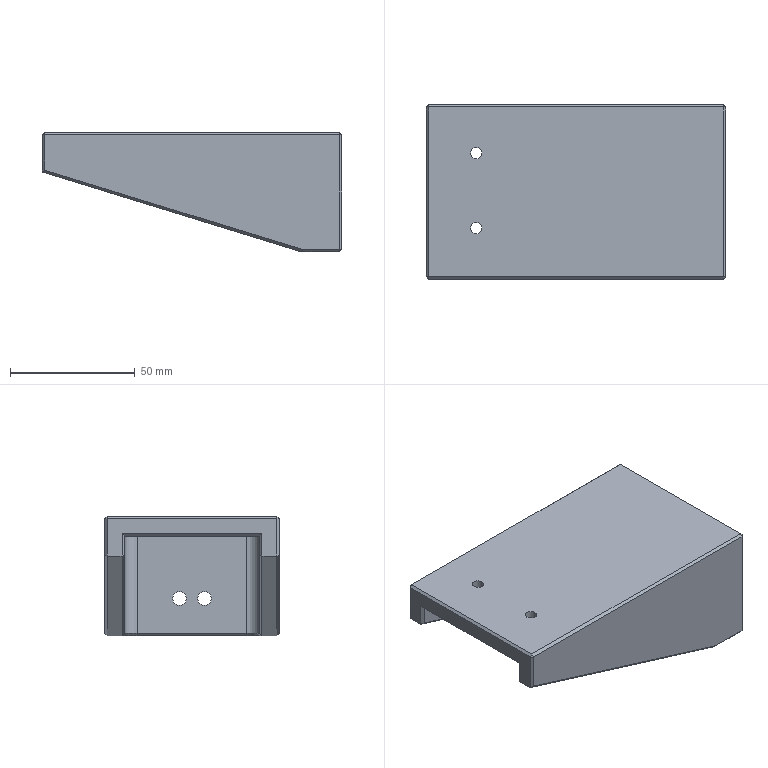Part | 1 solid | 47 faces | box 120 x 70 x 48 mm | volume 133864 mm3 | plane 39 | cylinder 6 | cone 2 | commonest cylinder face diameters 4.5 x2 5.5 x2 10 x2
STEP:
#1=CARTESIAN_POINT('',(44.15,35.,-47.));
#2=VERTEX_POINT('',#1);
#3=CARTESIAN_POINT('',(44.,34.,-48.));
#4=VERTEX_POINT('',#3);
#5=CARTESIAN_POINT('',(44.15,35.,-47.));
#6=CARTESIAN_POINT('',(44.,34.,-48.));
#7=B_SPLINE_CURVE_WITH_KNOTS('',1,(#5,#6),.UNSPECIFIED.,.F.,.F.,(2,2),(-0.7111,0.7111),.UNSPECIFIED.);
#8=EDGE_CURVE('',#2,#4,#7,.T.);
#9=ORIENTED_EDGE('',*,*,#8,.F.);
#10=CARTESIAN_POINT('',(59.,35.,-47.));
#11=VERTEX_POINT('',#10);
#12=CARTESIAN_POINT('',(51.575,35.,-47.));
#13=DIRECTION('',(-1.,0.,0.));
#14=VECTOR('',#13,1000.);
#15=LINE('',#12,#14);
#16=EDGE_CURVE('',#11,#2,#15,.T.);
#17=ORIENTED_EDGE('',*,*,#16,.F.);
#18=CARTESIAN_POINT('',(59.,34.,-48.));
#19=VERTEX_POINT('',#18);
#20=CARTESIAN_POINT('',(59.,34.5,-47.5));
#21=DIRECTION('',(0.,-0.7071,-0.7071));
#22=VECTOR('',#21,1000.);
#23=LINE('',#20,#22);
#24=EDGE_CURVE('',#11,#19,#23,.T.);
#25=ORIENTED_EDGE('',*,*,#24,.T.);
#26=CARTESIAN_POINT('',(51.5,34.,-48.));
#27=DIRECTION('',(-1.,0.,0.));
#28=VECTOR('',#27,1000.);
#29=LINE('',#26,#28);
#30=EDGE_CURVE('',#19,#4,#29,.T.);
#31=ORIENTED_EDGE('',*,*,#30,.T.);
#32=EDGE_LOOP('',(#9,#17,#25,#31));
#33=FACE_BOUND('',#32,.T.);
#34=CARTESIAN_POINT('',(-0.5,35.,-47.));
#35=DIRECTION('',(0.,-0.7071,0.7071));
#36=DIRECTION('',(-1.,0.,0.));
#37=AXIS2_PLACEMENT_3D('',#34,#35,#36);
#38=PLANE('',#37);
#39=ADVANCED_FACE('',(#33),#38,.F.);
#40=ORIENTED_EDGE('',*,*,#8,.T.);
#41=CARTESIAN_POINT('',(-60.,34.,-16.));
#42=VERTEX_POINT('',#41);
#43=CARTESIAN_POINT('',(-8.,34.,-32.));
#44=DIRECTION('',(-0.9558,0.,0.2941));
#45=VECTOR('',#44,1000.);
#46=LINE('',#43,#45);
#47=EDGE_CURVE('',#4,#42,#46,.T.);
#48=ORIENTED_EDGE('',*,*,#47,.T.);
#49=CARTESIAN_POINT('',(-59.,35.,-15.261));
#50=VERTEX_POINT('',#49);
#51=CARTESIAN_POINT('',(-59.,35.,-15.261));
#52=CARTESIAN_POINT('',(-60.,34.,-16.));
#53=B_SPLINE_CURVE_WITH_KNOTS('',1,(#51,#52),.UNSPECIFIED.,.F.,.F.,(2,2),(-0.7977,0.7977),.UNSPECIFIED.);
#54=EDGE_CURVE('',#50,#42,#53,.T.);
#55=ORIENTED_EDGE('',*,*,#54,.F.);
#56=CARTESIAN_POINT('',(-7.425,35.,-31.131));
#57=DIRECTION('',(-0.9558,0.,0.2941));
#58=VECTOR('',#57,1000.);
#59=LINE('',#56,#58);
#60=EDGE_CURVE('',#2,#50,#59,.T.);
#61=ORIENTED_EDGE('',*,*,#60,.F.);
#62=EDGE_LOOP('',(#40,#48,#55,#61));
#63=FACE_BOUND('',#62,.T.);
#64=CARTESIAN_POINT('',(-3.219,34.,-33.471));
#65=DIRECTION('',(-0.208,0.7071,-0.6758));
#66=DIRECTION('',(-0.9558,0.,0.2941));
#67=AXIS2_PLACEMENT_3D('',#64,#65,#66);
#68=PLANE('',#67);
#69=ADVANCED_FACE('',(#63),#68,.T.);
#70=CARTESIAN_POINT('',(-60.,34.,-1.));
#71=VERTEX_POINT('',#70);
#72=CARTESIAN_POINT('',(-60.,34.,-8.5));
#73=DIRECTION('',(0.,0.,-1.));
#74=VECTOR('',#73,1000.);
#75=LINE('',#72,#74);
#76=EDGE_CURVE('',#71,#42,#75,.T.);
#77=ORIENTED_EDGE('',*,*,#76,.F.);
#78=CARTESIAN_POINT('',(-59.,35.,-1.));
#79=VERTEX_POINT('',#78);
#80=CARTESIAN_POINT('',(-59.5,34.5,-1.));
#81=DIRECTION('',(-0.7071,-0.7071,0.));
#82=VECTOR('',#81,1000.);
#83=LINE('',#80,#82);
#84=EDGE_CURVE('',#79,#71,#83,.T.);
#85=ORIENTED_EDGE('',*,*,#84,.F.);
#86=CARTESIAN_POINT('',(-59.,35.,-8.131));
#87=DIRECTION('',(0.,0.,-1.));
#88=VECTOR('',#87,1000.);
#89=LINE('',#86,#88);
#90=EDGE_CURVE('',#79,#50,#89,.T.);
#91=ORIENTED_EDGE('',*,*,#90,.T.);
#92=ORIENTED_EDGE('',*,*,#54,.T.);
#93=EDGE_LOOP('',(#77,#85,#91,#92));
#94=FACE_BOUND('',#93,.T.);
#95=CARTESIAN_POINT('',(-59.,35.,-24.5));
#96=DIRECTION('',(-0.7071,0.7071,0.));
#97=DIRECTION('',(0.,0.,-1.));
#98=AXIS2_PLACEMENT_3D('',#95,#96,#97);
#99=PLANE('',#98);
#100=ADVANCED_FACE('',(#94),#99,.T.);
#101=ORIENTED_EDGE('',*,*,#84,.T.);
#102=CARTESIAN_POINT('',(-59.,34.,0.));
#103=VERTEX_POINT('',#102);
#104=CARTESIAN_POINT('',(-59.5,34.,-0.5));
#105=DIRECTION('',(-0.7071,0.,-0.7071));
#106=VECTOR('',#105,1000.);
#107=LINE('',#104,#106);
#108=EDGE_CURVE('',#103,#71,#107,.T.);
#109=ORIENTED_EDGE('',*,*,#108,.F.);
#110=CARTESIAN_POINT('',(-59.,34.5,-0.5));
#111=DIRECTION('',(0.,0.7071,-0.7071));
#112=VECTOR('',#111,1000.);
#113=LINE('',#110,#112);
#114=EDGE_CURVE('',#103,#79,#113,.T.);
#115=ORIENTED_EDGE('',*,*,#114,.T.);
#116=EDGE_LOOP('',(#101,#109,#115));
#117=FACE_BOUND('',#116,.T.);
#118=CARTESIAN_POINT('',(-59.333,34.333,-0.6667));
#119=DIRECTION('',(0.5774,-0.5774,-0.5774));
#120=DIRECTION('',(-0.4082,-0.8165,0.4082));
#121=AXIS2_PLACEMENT_3D('',#118,#119,#120);
#122=PLANE('',#121);
#123=ADVANCED_FACE('',(#117),#122,.F.);
#124=ORIENTED_EDGE('',*,*,#24,.F.);
#125=CARTESIAN_POINT('',(60.,34.,-47.));
#126=VERTEX_POINT('',#125);
#127=CARTESIAN_POINT('',(59.5,34.5,-47.));
#128=DIRECTION('',(-0.7071,0.7071,0.));
#129=VECTOR('',#128,1000.);
#130=LINE('',#127,#129);
#131=EDGE_CURVE('',#126,#11,#130,.T.);
#132=ORIENTED_EDGE('',*,*,#131,.F.);
#133=CARTESIAN_POINT('',(59.5,34.,-47.5));
#134=DIRECTION('',(-0.7071,0.,-0.7071));
#135=VECTOR('',#134,1000.);
#136=LINE('',#133,#135);
#137=EDGE_CURVE('',#126,#19,#136,.T.);
#138=ORIENTED_EDGE('',*,*,#137,.T.);
#139=EDGE_LOOP('',(#124,#132,#138));
#140=FACE_BOUND('',#139,.T.);
#141=CARTESIAN_POINT('',(59.333,34.333,-47.333));
#142=DIRECTION('',(-0.5774,-0.5774,0.5774));
#143=DIRECTION('',(0.4082,-0.8165,-0.4082));
#144=AXIS2_PLACEMENT_3D('',#141,#142,#143);
#145=PLANE('',#144);
#146=ADVANCED_FACE('',(#140),#145,.F.);
#147=CARTESIAN_POINT('',(-60.,-34.,-1.));
#148=VERTEX_POINT('',#147);
#149=CARTESIAN_POINT('',(-60.,0.,-1.));
#150=DIRECTION('',(0.,1.,0.));
#151=VECTOR('',#150,1000.);
#152=LINE('',#149,#151);
#153=EDGE_CURVE('',#148,#71,#152,.T.);
#154=ORIENTED_EDGE('',*,*,#153,.F.);
#155=CARTESIAN_POINT('',(-59.,-34.,0.));
#156=VERTEX_POINT('',#155);
#157=CARTESIAN_POINT('',(-59.5,-34.,-0.5));
#158=DIRECTION('',(0.7071,0.,0.7071));
#159=VECTOR('',#158,1000.);
#160=LINE('',#157,#159);
#161=EDGE_CURVE('',#148,#156,#160,.T.);
#162=ORIENTED_EDGE('',*,*,#161,.T.);
#163=CARTESIAN_POINT('',(-59.,0.,0.));
#164=DIRECTION('',(0.,1.,0.));
#165=VECTOR('',#164,1000.);
#166=LINE('',#163,#165);
#167=EDGE_CURVE('',#156,#103,#166,.T.);
#168=ORIENTED_EDGE('',*,*,#167,.T.);
#169=ORIENTED_EDGE('',*,*,#108,.T.);
#170=EDGE_LOOP('',(#154,#162,#168,#169));
#171=FACE_BOUND('',#170,.T.);
#172=CARTESIAN_POINT('',(-59.,0.,0.));
#173=DIRECTION('',(-0.7071,0.,0.7071));
#174=DIRECTION('',(0.,1.,0.));
#175=AXIS2_PLACEMENT_3D('',#172,#173,#174);
#176=PLANE('',#175);
#177=ADVANCED_FACE('',(#171),#176,.T.);
#178=CARTESIAN_POINT('',(-60.,28.,-16.));
#179=VERTEX_POINT('',#178);
#180=CARTESIAN_POINT('',(-60.,31.,-16.));
#181=DIRECTION('',(0.,-1.,0.));
#182=VECTOR('',#181,1000.);
#183=LINE('',#180,#182);
#184=EDGE_CURVE('',#42,#179,#183,.T.);
#185=ORIENTED_EDGE('',*,*,#184,.T.);
#186=CARTESIAN_POINT('',(-60.,28.,-7.));
#187=VERTEX_POINT('',#186);
#188=CARTESIAN_POINT('',(-60.,28.,-26.4));
#189=DIRECTION('',(0.,0.,1.));
#190=VECTOR('',#189,1000.);
#191=LINE('',#188,#190);
#192=EDGE_CURVE('',#179,#187,#191,.T.);
#193=ORIENTED_EDGE('',*,*,#192,.T.);
#194=CARTESIAN_POINT('',(-60.,-28.,-7.));
#195=VERTEX_POINT('',#194);
#196=CARTESIAN_POINT('',(-60.,0.,-7.));
#197=DIRECTION('',(0.,1.,0.));
#198=VECTOR('',#197,1000.);
#199=LINE('',#196,#198);
#200=EDGE_CURVE('',#195,#187,#199,.T.);
#201=ORIENTED_EDGE('',*,*,#200,.F.);
#202=CARTESIAN_POINT('',(-60.,-28.,-16.));
#203=VERTEX_POINT('',#202);
#204=CARTESIAN_POINT('',(-60.,-28.,-26.4));
#205=DIRECTION('',(0.,0.,1.));
#206=VECTOR('',#205,1000.);
#207=LINE('',#204,#206);
#208=EDGE_CURVE('',#203,#195,#207,.T.);
#209=ORIENTED_EDGE('',*,*,#208,.F.);
#210=CARTESIAN_POINT('',(-60.,-34.,-16.));
#211=VERTEX_POINT('',#210);
#212=CARTESIAN_POINT('',(-60.,-31.,-16.));
#213=DIRECTION('',(0.,1.,0.));
#214=VECTOR('',#213,1000.);
#215=LINE('',#212,#214);
#216=EDGE_CURVE('',#211,#203,#215,.T.);
#217=ORIENTED_EDGE('',*,*,#216,.F.);
#218=CARTESIAN_POINT('',(-60.,-34.,-24.5));
#219=DIRECTION('',(0.,0.,-1.));
#220=VECTOR('',#219,1000.);
#221=LINE('',#218,#220);
#222=EDGE_CURVE('',#148,#211,#221,.T.);
#223=ORIENTED_EDGE('',*,*,#222,.F.);
#224=ORIENTED_EDGE('',*,*,#153,.T.);
#225=ORIENTED_EDGE('',*,*,#76,.T.);
#226=EDGE_LOOP('',(#185,#193,#201,#209,#217,#223,#224,#225));
#227=FACE_BOUND('',#226,.T.);
#228=CARTESIAN_POINT('',(-60.,-35.,0.));
#229=DIRECTION('',(-1.,0.,0.));
#230=DIRECTION('',(0.,1.,0.));
#231=AXIS2_PLACEMENT_3D('',#228,#229,#230);
#232=PLANE('',#231);
#233=ADVANCED_FACE('',(#227),#232,.T.);
#234=CARTESIAN_POINT('',(59.,-34.,-48.));
#235=VERTEX_POINT('',#234);
#236=CARTESIAN_POINT('',(59.,0.,-48.));
#237=DIRECTION('',(0.,-1.,0.));
#238=VECTOR('',#237,1000.);
#239=LINE('',#236,#238);
#240=EDGE_CURVE('',#19,#235,#239,.T.);
#241=ORIENTED_EDGE('',*,*,#240,.T.);
#242=CARTESIAN_POINT('',(44.,-34.,-48.));
#243=VERTEX_POINT('',#242);
#244=CARTESIAN_POINT('',(-0.5,-34.,-48.));
#245=DIRECTION('',(1.,0.,0.));
#246=VECTOR('',#245,1000.);
#247=LINE('',#244,#246);
#248=EDGE_CURVE('',#243,#235,#247,.T.);
#249=ORIENTED_EDGE('',*,*,#248,.F.);
#250=CARTESIAN_POINT('',(44.,-28.,-48.));
#251=VERTEX_POINT('',#250);
#252=CARTESIAN_POINT('',(44.,-31.,-48.));
#253=DIRECTION('',(0.,1.,0.));
#254=VECTOR('',#253,1000.);
#255=LINE('',#252,#254);
#256=EDGE_CURVE('',#243,#251,#255,.T.);
#257=ORIENTED_EDGE('',*,*,#256,.T.);
#258=CARTESIAN_POINT('',(47.,-28.,-48.));
#259=VERTEX_POINT('',#258);
#260=CARTESIAN_POINT('',(-6.5,-28.,-48.));
#261=DIRECTION('',(-1.,0.,0.));
#262=VECTOR('',#261,1000.);
#263=LINE('',#260,#262);
#264=EDGE_CURVE('',#259,#251,#263,.T.);
#265=ORIENTED_EDGE('',*,*,#264,.F.);
#266=CARTESIAN_POINT('',(53.,-22.,-48.));
#267=VERTEX_POINT('',#266);
#268=CARTESIAN_POINT('',(47.,-22.,-48.));
#269=DIRECTION('',(0.,0.,-1.));
#270=DIRECTION('',(1.,0.,0.));
#271=AXIS2_PLACEMENT_3D('',#268,#269,#270);
#272=CIRCLE('',#271,6.);
#273=EDGE_CURVE('',#267,#259,#272,.T.);
#274=ORIENTED_EDGE('',*,*,#273,.F.);
#275=CARTESIAN_POINT('',(53.,22.,-48.));
#276=VERTEX_POINT('',#275);
#277=CARTESIAN_POINT('',(53.,0.,-48.));
#278=DIRECTION('',(0.,1.,0.));
#279=VECTOR('',#278,1000.);
#280=LINE('',#277,#279);
#281=EDGE_CURVE('',#267,#276,#280,.T.);
#282=ORIENTED_EDGE('',*,*,#281,.T.);
#283=CARTESIAN_POINT('',(47.,28.,-48.));
#284=VERTEX_POINT('',#283);
#285=CARTESIAN_POINT('',(47.,22.,-48.));
#286=DIRECTION('',(0.,0.,-1.));
#287=DIRECTION('',(1.,0.,0.));
#288=AXIS2_PLACEMENT_3D('',#285,#286,#287);
#289=CIRCLE('',#288,6.);
#290=EDGE_CURVE('',#284,#276,#289,.T.);
#291=ORIENTED_EDGE('',*,*,#290,.F.);
#292=CARTESIAN_POINT('',(44.,28.,-48.));
#293=VERTEX_POINT('',#292);
#294=CARTESIAN_POINT('',(-6.5,28.,-48.));
#295=DIRECTION('',(-1.,0.,0.));
#296=VECTOR('',#295,1000.);
#297=LINE('',#294,#296);
#298=EDGE_CURVE('',#284,#293,#297,.T.);
#299=ORIENTED_EDGE('',*,*,#298,.T.);
#300=CARTESIAN_POINT('',(44.,31.,-48.));
#301=DIRECTION('',(0.,-1.,0.));
#302=VECTOR('',#301,1000.);
#303=LINE('',#300,#302);
#304=EDGE_CURVE('',#4,#293,#303,.T.);
#305=ORIENTED_EDGE('',*,*,#304,.F.);
#306=ORIENTED_EDGE('',*,*,#30,.F.);
#307=EDGE_LOOP('',(#241,#249,#257,#265,#274,#282,#291,#299,#305,#306));
#308=FACE_BOUND('',#307,.T.);
#309=CARTESIAN_POINT('',(60.,35.,-48.));
#310=DIRECTION('',(0.,0.,-1.));
#311=DIRECTION('',(1.,0.,0.));
#312=AXIS2_PLACEMENT_3D('',#309,#310,#311);
#313=PLANE('',#312);
#314=ADVANCED_FACE('',(#308),#313,.T.);
#315=CARTESIAN_POINT('',(60.,-34.,-47.));
#316=VERTEX_POINT('',#315);
#317=CARTESIAN_POINT('',(60.,0.,-47.));
#318=DIRECTION('',(0.,-1.,0.));
#319=VECTOR('',#318,1000.);
#320=LINE('',#317,#319);
#321=EDGE_CURVE('',#126,#316,#320,.T.);
#322=ORIENTED_EDGE('',*,*,#321,.T.);
#323=CARTESIAN_POINT('',(59.5,-34.,-47.5));
#324=DIRECTION('',(0.7071,0.,0.7071));
#325=VECTOR('',#324,1000.);
#326=LINE('',#323,#325);
#327=EDGE_CURVE('',#235,#316,#326,.T.);
#328=ORIENTED_EDGE('',*,*,#327,.F.);
#329=ORIENTED_EDGE('',*,*,#240,.F.);
#330=ORIENTED_EDGE('',*,*,#137,.F.);
#331=EDGE_LOOP('',(#322,#328,#329,#330));
#332=FACE_BOUND('',#331,.T.);
#333=CARTESIAN_POINT('',(60.,0.,-47.));
#334=DIRECTION('',(0.7071,0.,-0.7071));
#335=DIRECTION('',(0.,-1.,0.));
#336=AXIS2_PLACEMENT_3D('',#333,#334,#335);
#337=PLANE('',#336);
#338=ADVANCED_FACE('',(#332),#337,.T.);
#339=ORIENTED_EDGE('',*,*,#114,.F.);
#340=CARTESIAN_POINT('',(59.,34.,0.));
#341=VERTEX_POINT('',#340);
#342=CARTESIAN_POINT('',(0.,34.,0.));
#343=DIRECTION('',(-1.,0.,0.));
#344=VECTOR('',#343,1000.);
#345=LINE('',#342,#344);
#346=EDGE_CURVE('',#341,#103,#345,.T.);
#347=ORIENTED_EDGE('',*,*,#346,.F.);
#348=CARTESIAN_POINT('',(59.,35.,-1.));
#349=VERTEX_POINT('',#348);
#350=CARTESIAN_POINT('',(59.,34.5,-0.5));
#351=DIRECTION('',(0.,0.7071,-0.7071));
#352=VECTOR('',#351,1000.);
#353=LINE('',#350,#352);
#354=EDGE_CURVE('',#341,#349,#353,.T.);
#355=ORIENTED_EDGE('',*,*,#354,.T.);
#356=CARTESIAN_POINT('',(0.,35.,-1.));
#357=DIRECTION('',(-1.,0.,0.));
#358=VECTOR('',#357,1000.);
#359=LINE('',#356,#358);
#360=EDGE_CURVE('',#349,#79,#359,.T.);
#361=ORIENTED_EDGE('',*,*,#360,.T.);
#362=EDGE_LOOP('',(#339,#347,#355,#361));
#363=FACE_BOUND('',#362,.T.);
#364=CARTESIAN_POINT('',(-0.5,34.,0.));
#365=DIRECTION('',(0.,-0.7071,-0.7071));
#366=DIRECTION('',(-1.,0.,0.));
#367=AXIS2_PLACEMENT_3D('',#364,#365,#366);
#368=PLANE('',#367);
#369=ADVANCED_FACE('',(#363),#368,.F.);
#370=CARTESIAN_POINT('',(59.,35.,-24.));
#371=DIRECTION('',(0.,0.,-1.));
#372=VECTOR('',#371,1000.);
#373=LINE('',#370,#372);
#374=EDGE_CURVE('',#349,#11,#373,.T.);
#375=ORIENTED_EDGE('',*,*,#374,.F.);
#376=CARTESIAN_POINT('',(60.,34.,-1.));
#377=VERTEX_POINT('',#376);
#378=CARTESIAN_POINT('',(59.5,34.5,-1.));
#379=DIRECTION('',(0.7071,-0.7071,0.));
#380=VECTOR('',#379,1000.);
#381=LINE('',#378,#380);
#382=EDGE_CURVE('',#349,#377,#381,.T.);
#383=ORIENTED_EDGE('',*,*,#382,.T.);
#384=CARTESIAN_POINT('',(60.,34.,-24.));
#385=DIRECTION('',(0.,0.,-1.));
#386=VECTOR('',#385,1000.);
#387=LINE('',#384,#386);
#388=EDGE_CURVE('',#377,#126,#387,.T.);
#389=ORIENTED_EDGE('',*,*,#388,.T.);
#390=ORIENTED_EDGE('',*,*,#131,.T.);
#391=EDGE_LOOP('',(#375,#383,#389,#390));
#392=FACE_BOUND('',#391,.T.);
#393=CARTESIAN_POINT('',(60.,34.,-24.));
#394=DIRECTION('',(0.7071,0.7071,0.));
#395=DIRECTION('',(0.,0.,-1.));
#396=AXIS2_PLACEMENT_3D('',#393,#394,#395);
#397=PLANE('',#396);
#398=ADVANCED_FACE('',(#392),#397,.T.);
#399=ORIENTED_EDGE('',*,*,#16,.T.);
#400=ORIENTED_EDGE('',*,*,#60,.T.);
#401=ORIENTED_EDGE('',*,*,#90,.F.);
#402=ORIENTED_EDGE('',*,*,#360,.F.);
#403=ORIENTED_EDGE('',*,*,#374,.T.);
#404=EDGE_LOOP('',(#399,#400,#401,#402,#403));
#405=FACE_BOUND('',#404,.T.);
#406=CARTESIAN_POINT('',(60.,35.,0.));
#407=DIRECTION('',(0.,-1.,0.));
#408=DIRECTION('',(-1.,0.,0.));
#409=AXIS2_PLACEMENT_3D('',#406,#407,#408);
#410=PLANE('',#409);
#411=ADVANCED_FACE('',(#405),#410,.F.);
#412=ORIENTED_EDGE('',*,*,#47,.F.);
#413=ORIENTED_EDGE('',*,*,#304,.T.);
#414=CARTESIAN_POINT('',(-6.794,28.,-32.371));
#415=DIRECTION('',(-0.9558,0.,0.2941));
#416=VECTOR('',#415,1000.);
#417=LINE('',#414,#416);
#418=EDGE_CURVE('',#293,#179,#417,.T.);
#419=ORIENTED_EDGE('',*,*,#418,.T.);
#420=ORIENTED_EDGE('',*,*,#184,.F.);
#421=EDGE_LOOP('',(#412,#413,#419,#420));
#422=FACE_BOUND('',#421,.T.);
#423=CARTESIAN_POINT('',(44.,35.,-48.));
#424=DIRECTION('',(0.2941,0.,0.9558));
#425=DIRECTION('',(-0.9558,0.,0.2941));
#426=AXIS2_PLACEMENT_3D('',#423,#424,#425);
#427=PLANE('',#426);
#428=ADVANCED_FACE('',(#422),#427,.F.);
#429=CARTESIAN_POINT('',(44.15,-35.,-47.));
#430=VERTEX_POINT('',#429);
#431=CARTESIAN_POINT('',(44.,-34.,-48.));
#432=CARTESIAN_POINT('',(44.15,-35.,-47.));
#433=B_SPLINE_CURVE_WITH_KNOTS('',1,(#431,#432),.UNSPECIFIED.,.F.,.F.,(2,2),(-0.7111,0.7111),.UNSPECIFIED.);
#434=EDGE_CURVE('',#243,#430,#433,.T.);
#435=ORIENTED_EDGE('',*,*,#434,.F.);
#436=ORIENTED_EDGE('',*,*,#248,.T.);
#437=CARTESIAN_POINT('',(59.,-35.,-47.));
#438=VERTEX_POINT('',#437);
#439=CARTESIAN_POINT('',(59.,-34.5,-47.5));
#440=DIRECTION('',(0.,0.7071,-0.7071));
#441=VECTOR('',#440,1000.);
#442=LINE('',#439,#441);
#443=EDGE_CURVE('',#438,#235,#442,.T.);
#444=ORIENTED_EDGE('',*,*,#443,.F.);
#445=CARTESIAN_POINT('',(51.575,-35.,-47.));
#446=DIRECTION('',(1.,0.,0.));
#447=VECTOR('',#446,1000.);
#448=LINE('',#445,#447);
#449=EDGE_CURVE('',#430,#438,#448,.T.);
#450=ORIENTED_EDGE('',*,*,#449,.F.);
#451=EDGE_LOOP('',(#435,#436,#444,#450));
#452=FACE_BOUND('',#451,.T.);
#453=CARTESIAN_POINT('',(-0.5,-35.,-47.));
#454=DIRECTION('',(0.,0.7071,0.7071));
#455=DIRECTION('',(1.,0.,0.));
#456=AXIS2_PLACEMENT_3D('',#453,#454,#455);
#457=PLANE('',#456);
#458=ADVANCED_FACE('',(#452),#457,.F.);
#459=CARTESIAN_POINT('',(-59.,-35.,-15.261));
#460=VERTEX_POINT('',#459);
#461=CARTESIAN_POINT('',(-7.425,-35.,-31.131));
#462=DIRECTION('',(-0.9558,0.,0.2941));
#463=VECTOR('',#462,1000.);
#464=LINE('',#461,#463);
#465=EDGE_CURVE('',#430,#460,#464,.T.);
#466=ORIENTED_EDGE('',*,*,#465,.T.);
#467=CARTESIAN_POINT('',(-60.,-34.,-16.));
#468=CARTESIAN_POINT('',(-59.,-35.,-15.261));
#469=B_SPLINE_CURVE_WITH_KNOTS('',1,(#467,#468),.UNSPECIFIED.,.F.,.F.,(2,2),(-0.7977,0.7977),.UNSPECIFIED.);
#470=EDGE_CURVE('',#211,#460,#469,.T.);
#471=ORIENTED_EDGE('',*,*,#470,.F.);
#472=CARTESIAN_POINT('',(-8.,-34.,-32.));
#473=DIRECTION('',(-0.9558,0.,0.2941));
#474=VECTOR('',#473,1000.);
#475=LINE('',#472,#474);
#476=EDGE_CURVE('',#243,#211,#475,.T.);
#477=ORIENTED_EDGE('',*,*,#476,.F.);
#478=ORIENTED_EDGE('',*,*,#434,.T.);
#479=EDGE_LOOP('',(#466,#471,#477,#478));
#480=FACE_BOUND('',#479,.T.);
#481=CARTESIAN_POINT('',(-3.219,-34.,-33.471));
#482=DIRECTION('',(0.208,0.7071,0.6758));
#483=DIRECTION('',(-0.9558,0.,0.2941));
#484=AXIS2_PLACEMENT_3D('',#481,#482,#483);
#485=PLANE('',#484);
#486=ADVANCED_FACE('',(#480),#485,.F.);
#487=CARTESIAN_POINT('',(-59.,-35.,-1.));
#488=VERTEX_POINT('',#487);
#489=CARTESIAN_POINT('',(-59.,-35.,-8.131));
#490=DIRECTION('',(0.,0.,-1.));
#491=VECTOR('',#490,1000.);
#492=LINE('',#489,#491);
#493=EDGE_CURVE('',#488,#460,#492,.T.);
#494=ORIENTED_EDGE('',*,*,#493,.F.);
#495=CARTESIAN_POINT('',(-59.5,-34.5,-1.));
#496=DIRECTION('',(0.7071,-0.7071,0.));
#497=VECTOR('',#496,1000.);
#498=LINE('',#495,#497);
#499=EDGE_CURVE('',#148,#488,#498,.T.);
#500=ORIENTED_EDGE('',*,*,#499,.F.);
#501=ORIENTED_EDGE('',*,*,#222,.T.);
#502=ORIENTED_EDGE('',*,*,#470,.T.);
#503=EDGE_LOOP('',(#494,#500,#501,#502));
#504=FACE_BOUND('',#503,.T.);
#505=CARTESIAN_POINT('',(-60.,-34.,-24.5));
#506=DIRECTION('',(-0.7071,-0.7071,0.));
#507=DIRECTION('',(0.,0.,-1.));
#508=AXIS2_PLACEMENT_3D('',#505,#506,#507);
#509=PLANE('',#508);
#510=ADVANCED_FACE('',(#504),#509,.T.);
#511=ORIENTED_EDGE('',*,*,#499,.T.);
#512=CARTESIAN_POINT('',(-59.,-34.5,-0.5));
#513=DIRECTION('',(0.,-0.7071,-0.7071));
#514=VECTOR('',#513,1000.);
#515=LINE('',#512,#514);
#516=EDGE_CURVE('',#156,#488,#515,.T.);
#517=ORIENTED_EDGE('',*,*,#516,.F.);
#518=ORIENTED_EDGE('',*,*,#161,.F.);
#519=EDGE_LOOP('',(#511,#517,#518));
#520=FACE_BOUND('',#519,.T.);
#521=CARTESIAN_POINT('',(-59.333,-34.333,-0.6667));
#522=DIRECTION('',(0.5774,0.5774,-0.5774));
#523=DIRECTION('',(0.4082,-0.8165,-0.4082));
#524=AXIS2_PLACEMENT_3D('',#521,#522,#523);
#525=PLANE('',#524);
#526=ADVANCED_FACE('',(#520),#525,.F.);
#527=ORIENTED_EDGE('',*,*,#443,.T.);
#528=ORIENTED_EDGE('',*,*,#327,.T.);
#529=CARTESIAN_POINT('',(59.5,-34.5,-47.));
#530=DIRECTION('',(0.7071,0.7071,0.));
#531=VECTOR('',#530,1000.);
#532=LINE('',#529,#531);
#533=EDGE_CURVE('',#438,#316,#532,.T.);
#534=ORIENTED_EDGE('',*,*,#533,.F.);
#535=EDGE_LOOP('',(#527,#528,#534));
#536=FACE_BOUND('',#535,.T.);
#537=CARTESIAN_POINT('',(59.333,-34.333,-47.333));
#538=DIRECTION('',(0.5774,-0.5774,-0.5774));
#539=DIRECTION('',(-0.4082,-0.8165,0.4082));
#540=AXIS2_PLACEMENT_3D('',#537,#538,#539);
#541=PLANE('',#540);
#542=ADVANCED_FACE('',(#536),#541,.T.);
#543=ORIENTED_EDGE('',*,*,#516,.T.);
#544=CARTESIAN_POINT('',(59.,-35.,-1.));
#545=VERTEX_POINT('',#544);
#546=CARTESIAN_POINT('',(0.,-35.,-1.));
#547=DIRECTION('',(1.,0.,0.));
#548=VECTOR('',#547,1000.);
#549=LINE('',#546,#548);
#550=EDGE_CURVE('',#488,#545,#549,.T.);
#551=ORIENTED_EDGE('',*,*,#550,.T.);
#552=CARTESIAN_POINT('',(59.,-34.,0.));
#553=VERTEX_POINT('',#552);
#554=CARTESIAN_POINT('',(59.,-34.5,-0.5));
#555=DIRECTION('',(0.,-0.7071,-0.7071));
#556=VECTOR('',#555,1000.);
#557=LINE('',#554,#556);
#558=EDGE_CURVE('',#553,#545,#557,.T.);
#559=ORIENTED_EDGE('',*,*,#558,.F.);
#560=CARTESIAN_POINT('',(0.,-34.,0.));
#561=DIRECTION('',(1.,0.,0.));
#562=VECTOR('',#561,1000.);
#563=LINE('',#560,#562);
#564=EDGE_CURVE('',#156,#553,#563,.T.);
#565=ORIENTED_EDGE('',*,*,#564,.F.);
#566=EDGE_LOOP('',(#543,#551,#559,#565));
#567=FACE_BOUND('',#566,.T.);
#568=CARTESIAN_POINT('',(-0.5,-34.,0.));
#569=DIRECTION('',(0.,0.7071,-0.7071));
#570=DIRECTION('',(1.,0.,0.));
#571=AXIS2_PLACEMENT_3D('',#568,#569,#570);
#572=PLANE('',#571);
#573=ADVANCED_FACE('',(#567),#572,.F.);
#574=ORIENTED_EDGE('',*,*,#493,.T.);
#575=ORIENTED_EDGE('',*,*,#465,.F.);
#576=ORIENTED_EDGE('',*,*,#449,.T.);
#577=CARTESIAN_POINT('',(59.,-35.,-24.));
#578=DIRECTION('',(0.,0.,-1.));
#579=VECTOR('',#578,1000.);
#580=LINE('',#577,#579);
#581=EDGE_CURVE('',#545,#438,#580,.T.);
#582=ORIENTED_EDGE('',*,*,#581,.F.);
#583=ORIENTED_EDGE('',*,*,#550,.F.);
#584=EDGE_LOOP('',(#574,#575,#576,#582,#583));
#585=FACE_BOUND('',#584,.T.);
#586=CARTESIAN_POINT('',(-60.,-35.,0.));
#587=DIRECTION('',(0.,1.,0.));
#588=DIRECTION('',(1.,0.,0.));
#589=AXIS2_PLACEMENT_3D('',#586,#587,#588);
#590=PLANE('',#589);
#591=ADVANCED_FACE('',(#585),#590,.F.);
#592=CARTESIAN_POINT('',(60.,-34.,-1.));
#593=VERTEX_POINT('',#592);
#594=CARTESIAN_POINT('',(60.,-34.,-24.));
#595=DIRECTION('',(0.,0.,-1.));
#596=VECTOR('',#595,1000.);
#597=LINE('',#594,#596);
#598=EDGE_CURVE('',#593,#316,#597,.T.);
#599=ORIENTED_EDGE('',*,*,#598,.F.);
#600=CARTESIAN_POINT('',(59.5,-34.5,-1.));
#601=DIRECTION('',(0.7071,0.7071,0.));
#602=VECTOR('',#601,1000.);
#603=LINE('',#600,#602);
#604=EDGE_CURVE('',#545,#593,#603,.T.);
#605=ORIENTED_EDGE('',*,*,#604,.F.);
#606=ORIENTED_EDGE('',*,*,#581,.T.);
#607=ORIENTED_EDGE('',*,*,#533,.T.);
#608=EDGE_LOOP('',(#599,#605,#606,#607));
#609=FACE_BOUND('',#608,.T.);
#610=CARTESIAN_POINT('',(59.,-35.,-24.));
#611=DIRECTION('',(0.7071,-0.7071,0.));
#612=DIRECTION('',(0.,0.,-1.));
#613=AXIS2_PLACEMENT_3D('',#610,#611,#612);
#614=PLANE('',#613);
#615=ADVANCED_FACE('',(#609),#614,.T.);
#616=ORIENTED_EDGE('',*,*,#476,.T.);
#617=ORIENTED_EDGE('',*,*,#216,.T.);
#618=CARTESIAN_POINT('',(-6.794,-28.,-32.371));
#619=DIRECTION('',(-0.9558,0.,0.2941));
#620=VECTOR('',#619,1000.);
#621=LINE('',#618,#620);
#622=EDGE_CURVE('',#251,#203,#621,.T.);
#623=ORIENTED_EDGE('',*,*,#622,.F.);
#624=ORIENTED_EDGE('',*,*,#256,.F.);
#625=EDGE_LOOP('',(#616,#617,#623,#624));
#626=FACE_BOUND('',#625,.T.);
#627=CARTESIAN_POINT('',(44.,35.,-48.));
#628=DIRECTION('',(0.2941,0.,0.9558));
#629=DIRECTION('',(-0.9558,0.,0.2941));
#630=AXIS2_PLACEMENT_3D('',#627,#628,#629);
#631=PLANE('',#630);
#632=ADVANCED_FACE('',(#626),#631,.F.);
#633=ORIENTED_EDGE('',*,*,#558,.T.);
#634=ORIENTED_EDGE('',*,*,#604,.T.);
#635=CARTESIAN_POINT('',(59.5,-34.,-0.5));
#636=DIRECTION('',(0.7071,0.,-0.7071));
#637=VECTOR('',#636,1000.);
#638=LINE('',#635,#637);
#639=EDGE_CURVE('',#553,#593,#638,.T.);
#640=ORIENTED_EDGE('',*,*,#639,.F.);
#641=EDGE_LOOP('',(#633,#634,#640));
#642=FACE_BOUND('',#641,.T.);
#643=CARTESIAN_POINT('',(59.333,-34.333,-0.6667));
#644=DIRECTION('',(-0.5774,0.5774,-0.5774));
#645=DIRECTION('',(-0.4082,-0.8165,-0.4082));
#646=AXIS2_PLACEMENT_3D('',#643,#644,#645);
#647=PLANE('',#646);
#648=ADVANCED_FACE('',(#642),#647,.F.);
#649=CARTESIAN_POINT('',(-37.75,-14.5,0.));
#650=VERTEX_POINT('',#649);
#651=CARTESIAN_POINT('',(-40.,-14.5,0.));
#652=DIRECTION('',(0.,0.,-1.));
#653=DIRECTION('',(1.,0.,0.));
#654=AXIS2_PLACEMENT_3D('',#651,#652,#653);
#655=CIRCLE('',#654,2.25);
#656=EDGE_CURVE('',#650,#650,#655,.T.);
#657=ORIENTED_EDGE('',*,*,#656,.T.);
#658=EDGE_LOOP('',(#657));
#659=FACE_BOUND('',#658,.T.);
#660=CARTESIAN_POINT('',(-37.75,15.5,0.));
#661=VERTEX_POINT('',#660);
#662=CARTESIAN_POINT('',(-40.,15.5,0.));
#663=DIRECTION('',(0.,0.,-1.));
#664=DIRECTION('',(1.,0.,0.));
#665=AXIS2_PLACEMENT_3D('',#662,#663,#664);
#666=CIRCLE('',#665,2.25);
#667=EDGE_CURVE('',#661,#661,#666,.T.);
#668=ORIENTED_EDGE('',*,*,#667,.T.);
#669=EDGE_LOOP('',(#668));
#670=FACE_BOUND('',#669,.T.);
#671=ORIENTED_EDGE('',*,*,#564,.T.);
#672=CARTESIAN_POINT('',(59.,0.,0.));
#673=DIRECTION('',(0.,-1.,0.));
#674=VECTOR('',#673,1000.);
#675=LINE('',#672,#674);
#676=EDGE_CURVE('',#341,#553,#675,.T.);
#677=ORIENTED_EDGE('',*,*,#676,.F.);
#678=ORIENTED_EDGE('',*,*,#346,.T.);
#679=ORIENTED_EDGE('',*,*,#167,.F.);
#680=EDGE_LOOP('',(#671,#677,#678,#679));
#681=FACE_BOUND('',#680,.T.);
#682=CARTESIAN_POINT('',(60.,35.,0.));
#683=DIRECTION('',(0.,0.,-1.));
#684=DIRECTION('',(1.,0.,0.));
#685=AXIS2_PLACEMENT_3D('',#682,#683,#684);
#686=PLANE('',#685);
#687=ADVANCED_FACE('',(#659,#670,#681),#686,.F.);
#688=CARTESIAN_POINT('',(60.,0.,-1.));
#689=DIRECTION('',(0.,-1.,0.));
#690=VECTOR('',#689,1000.);
#691=LINE('',#688,#690);
#692=EDGE_CURVE('',#377,#593,#691,.T.);
#693=ORIENTED_EDGE('',*,*,#692,.F.);
#694=CARTESIAN_POINT('',(59.5,34.,-0.5));
#695=DIRECTION('',(0.7071,0.,-0.7071));
#696=VECTOR('',#695,1000.);
#697=LINE('',#694,#696);
#698=EDGE_CURVE('',#341,#377,#697,.T.);
#699=ORIENTED_EDGE('',*,*,#698,.F.);
#700=ORIENTED_EDGE('',*,*,#676,.T.);
#701=ORIENTED_EDGE('',*,*,#639,.T.);
#702=EDGE_LOOP('',(#693,#699,#700,#701));
#703=FACE_BOUND('',#702,.T.);
#704=CARTESIAN_POINT('',(59.,0.,0.));
#705=DIRECTION('',(0.7071,0.,0.7071));
#706=DIRECTION('',(0.,-1.,0.));
#707=AXIS2_PLACEMENT_3D('',#704,#705,#706);
#708=PLANE('',#707);
#709=ADVANCED_FACE('',(#703),#708,.T.);
#710=ORIENTED_EDGE('',*,*,#354,.F.);
#711=ORIENTED_EDGE('',*,*,#698,.T.);
#712=ORIENTED_EDGE('',*,*,#382,.F.);
#713=EDGE_LOOP('',(#710,#711,#712));
#714=FACE_BOUND('',#713,.T.);
#715=CARTESIAN_POINT('',(59.333,34.333,-0.6667));
#716=DIRECTION('',(-0.5774,-0.5774,-0.5774));
#717=DIRECTION('',(0.4082,-0.8165,0.4082));
#718=AXIS2_PLACEMENT_3D('',#715,#716,#717);
#719=PLANE('',#718);
#720=ADVANCED_FACE('',(#714),#719,.F.);
#721=CARTESIAN_POINT('',(-59.,27.,-8.));
#722=VERTEX_POINT('',#721);
#723=CARTESIAN_POINT('',(-59.,27.,-8.));
#724=CARTESIAN_POINT('',(-60.,28.,-7.));
#725=B_SPLINE_CURVE_WITH_KNOTS('',1,(#723,#724),.UNSPECIFIED.,.F.,.F.,(2,2),(-0.866,0.866),.UNSPECIFIED.);
#726=EDGE_CURVE('',#722,#187,#725,.T.);
#727=ORIENTED_EDGE('',*,*,#726,.T.);
#728=ORIENTED_EDGE('',*,*,#192,.F.);
#729=CARTESIAN_POINT('',(-59.,27.,-15.261));
#730=VERTEX_POINT('',#729);
#731=CARTESIAN_POINT('',(-59.,27.,-15.261));
#732=CARTESIAN_POINT('',(-60.,28.,-16.));
#733=B_SPLINE_CURVE_WITH_KNOTS('',1,(#731,#732),.UNSPECIFIED.,.F.,.F.,(2,2),(-0.7977,0.7977),.UNSPECIFIED.);
#734=EDGE_CURVE('',#730,#179,#733,.T.);
#735=ORIENTED_EDGE('',*,*,#734,.F.);
#736=CARTESIAN_POINT('',(-59.,27.,-11.631));
#737=DIRECTION('',(0.,0.,1.));
#738=VECTOR('',#737,1000.);
#739=LINE('',#736,#738);
#740=EDGE_CURVE('',#730,#722,#739,.T.);
#741=ORIENTED_EDGE('',*,*,#740,.T.);
#742=EDGE_LOOP('',(#727,#728,#735,#741));
#743=FACE_BOUND('',#742,.T.);
#744=CARTESIAN_POINT('',(-59.,27.,-26.4));
#745=DIRECTION('',(-0.7071,-0.7071,0.));
#746=DIRECTION('',(0.,0.,1.));
#747=AXIS2_PLACEMENT_3D('',#744,#745,#746);
#748=PLANE('',#747);
#749=ADVANCED_FACE('',(#743),#748,.T.);
#750=ORIENTED_EDGE('',*,*,#734,.T.);
#751=ORIENTED_EDGE('',*,*,#418,.F.);
#752=CARTESIAN_POINT('',(44.15,27.,-47.));
#753=VERTEX_POINT('',#752);
#754=CARTESIAN_POINT('',(44.15,27.,-47.));
#755=CARTESIAN_POINT('',(44.,28.,-48.));
#756=B_SPLINE_CURVE_WITH_KNOTS('',1,(#754,#755),.UNSPECIFIED.,.F.,.F.,(2,2),(-0.7111,0.7111),.UNSPECIFIED.);
#757=EDGE_CURVE('',#753,#293,#756,.T.);
#758=ORIENTED_EDGE('',*,*,#757,.F.);
#759=CARTESIAN_POINT('',(-7.425,27.,-31.131));
#760=DIRECTION('',(-0.9558,0.,0.2941));
#761=VECTOR('',#760,1000.);
#762=LINE('',#759,#761);
#763=EDGE_CURVE('',#753,#730,#762,.T.);
#764=ORIENTED_EDGE('',*,*,#763,.T.);
#765=EDGE_LOOP('',(#750,#751,#758,#764));
#766=FACE_BOUND('',#765,.T.);
#767=CARTESIAN_POINT('',(-6.5,27.,-31.415));
#768=DIRECTION('',(-0.208,-0.7071,-0.6758));
#769=DIRECTION('',(-0.9558,0.,0.2941));
#770=AXIS2_PLACEMENT_3D('',#767,#768,#769);
#771=PLANE('',#770);
#772=ADVANCED_FACE('',(#766),#771,.T.);
#773=CARTESIAN_POINT('',(44.15,-27.,-47.));
#774=VERTEX_POINT('',#773);
#775=CARTESIAN_POINT('',(44.15,-27.,-47.));
#776=CARTESIAN_POINT('',(44.,-28.,-48.));
#777=B_SPLINE_CURVE_WITH_KNOTS('',1,(#775,#776),.UNSPECIFIED.,.F.,.F.,(2,2),(-0.7111,0.7111),.UNSPECIFIED.);
#778=EDGE_CURVE('',#774,#251,#777,.T.);
#779=ORIENTED_EDGE('',*,*,#778,.F.);
#780=CARTESIAN_POINT('',(47.,-27.,-47.));
#781=VERTEX_POINT('',#780);
#782=CARTESIAN_POINT('',(45.575,-27.,-47.));
#783=DIRECTION('',(-1.,0.,0.));
#784=VECTOR('',#783,1000.);
#785=LINE('',#782,#784);
#786=EDGE_CURVE('',#781,#774,#785,.T.);
#787=ORIENTED_EDGE('',*,*,#786,.F.);
#788=CARTESIAN_POINT('',(47.,-27.5,-47.5));
#789=DIRECTION('',(0.,-0.7071,-0.7071));
#790=VECTOR('',#789,1000.);
#791=LINE('',#788,#790);
#792=EDGE_CURVE('',#781,#259,#791,.T.);
#793=ORIENTED_EDGE('',*,*,#792,.T.);
#794=ORIENTED_EDGE('',*,*,#264,.T.);
#795=EDGE_LOOP('',(#779,#787,#793,#794));
#796=FACE_BOUND('',#795,.T.);
#797=CARTESIAN_POINT('',(-6.5,-27.,-47.));
#798=DIRECTION('',(0.,-0.7071,0.7071));
#799=DIRECTION('',(-1.,0.,0.));
#800=AXIS2_PLACEMENT_3D('',#797,#798,#799);
#801=PLANE('',#800);
#802=ADVANCED_FACE('',(#796),#801,.F.);
#803=ORIENTED_EDGE('',*,*,#298,.F.);
#804=CARTESIAN_POINT('',(47.,27.,-47.));
#805=VERTEX_POINT('',#804);
#806=CARTESIAN_POINT('',(47.,27.5,-47.5));
#807=DIRECTION('',(0.,0.7071,-0.7071));
#808=VECTOR('',#807,1000.);
#809=LINE('',#806,#808);
#810=EDGE_CURVE('',#805,#284,#809,.T.);
#811=ORIENTED_EDGE('',*,*,#810,.F.);
#812=CARTESIAN_POINT('',(45.575,27.,-47.));
#813=DIRECTION('',(-1.,0.,0.));
#814=VECTOR('',#813,1000.);
#815=LINE('',#812,#814);
#816=EDGE_CURVE('',#805,#753,#815,.T.);
#817=ORIENTED_EDGE('',*,*,#816,.T.);
#818=ORIENTED_EDGE('',*,*,#757,.T.);
#819=EDGE_LOOP('',(#803,#811,#817,#818));
#820=FACE_BOUND('',#819,.T.);
#821=CARTESIAN_POINT('',(-6.5,27.,-47.));
#822=DIRECTION('',(0.,-0.7071,-0.7071));
#823=DIRECTION('',(-1.,0.,0.));
#824=AXIS2_PLACEMENT_3D('',#821,#822,#823);
#825=PLANE('',#824);
#826=ADVANCED_FACE('',(#820),#825,.T.);
#827=ORIENTED_EDGE('',*,*,#622,.T.);
#828=CARTESIAN_POINT('',(-59.,-27.,-15.261));
#829=VERTEX_POINT('',#828);
#830=CARTESIAN_POINT('',(-59.,-27.,-15.261));
#831=CARTESIAN_POINT('',(-60.,-28.,-16.));
#832=B_SPLINE_CURVE_WITH_KNOTS('',1,(#830,#831),.UNSPECIFIED.,.F.,.F.,(2,2),(-0.7977,0.7977),.UNSPECIFIED.);
#833=EDGE_CURVE('',#829,#203,#832,.T.);
#834=ORIENTED_EDGE('',*,*,#833,.F.);
#835=CARTESIAN_POINT('',(-7.425,-27.,-31.131));
#836=DIRECTION('',(-0.9558,0.,0.2941));
#837=VECTOR('',#836,1000.);
#838=LINE('',#835,#837);
#839=EDGE_CURVE('',#774,#829,#838,.T.);
#840=ORIENTED_EDGE('',*,*,#839,.F.);
#841=ORIENTED_EDGE('',*,*,#778,.T.);
#842=EDGE_LOOP('',(#827,#834,#840,#841));
#843=FACE_BOUND('',#842,.T.);
#844=CARTESIAN_POINT('',(-6.5,-27.,-31.415));
#845=DIRECTION('',(0.208,-0.7071,0.6758));
#846=DIRECTION('',(-0.9558,0.,0.2941));
#847=AXIS2_PLACEMENT_3D('',#844,#845,#846);
#848=PLANE('',#847);
#849=ADVANCED_FACE('',(#843),#848,.F.);
#850=ORIENTED_EDGE('',*,*,#208,.T.);
#851=CARTESIAN_POINT('',(-59.,-27.,-8.));
#852=VERTEX_POINT('',#851);
#853=CARTESIAN_POINT('',(-59.,-27.,-8.));
#854=CARTESIAN_POINT('',(-60.,-28.,-7.));
#855=B_SPLINE_CURVE_WITH_KNOTS('',1,(#853,#854),.UNSPECIFIED.,.F.,.F.,(2,2),(-0.866,0.866),.UNSPECIFIED.);
#856=EDGE_CURVE('',#852,#195,#855,.T.);
#857=ORIENTED_EDGE('',*,*,#856,.F.);
#858=CARTESIAN_POINT('',(-59.,-27.,-11.631));
#859=DIRECTION('',(0.,0.,1.));
#860=VECTOR('',#859,1000.);
#861=LINE('',#858,#860);
#862=EDGE_CURVE('',#829,#852,#861,.T.);
#863=ORIENTED_EDGE('',*,*,#862,.F.);
#864=ORIENTED_EDGE('',*,*,#833,.T.);
#865=EDGE_LOOP('',(#850,#857,#863,#864));
#866=FACE_BOUND('',#865,.T.);
#867=CARTESIAN_POINT('',(-59.,-27.,-26.4));
#868=DIRECTION('',(0.7071,-0.7071,0.));
#869=DIRECTION('',(0.,0.,1.));
#870=AXIS2_PLACEMENT_3D('',#867,#868,#869);
#871=PLANE('',#870);
#872=ADVANCED_FACE('',(#866),#871,.F.);
#873=ORIENTED_EDGE('',*,*,#856,.T.);
#874=ORIENTED_EDGE('',*,*,#200,.T.);
#875=ORIENTED_EDGE('',*,*,#726,.F.);
#876=CARTESIAN_POINT('',(-59.,0.,-8.));
#877=DIRECTION('',(0.,1.,0.));
#878=VECTOR('',#877,1000.);
#879=LINE('',#876,#878);
#880=EDGE_CURVE('',#852,#722,#879,.T.);
#881=ORIENTED_EDGE('',*,*,#880,.F.);
#882=EDGE_LOOP('',(#873,#874,#875,#881));
#883=FACE_BOUND('',#882,.T.);
#884=CARTESIAN_POINT('',(-60.,0.,-7.));
#885=DIRECTION('',(-0.7071,0.,-0.7071));
#886=DIRECTION('',(0.,1.,0.));
#887=AXIS2_PLACEMENT_3D('',#884,#885,#886);
#888=PLANE('',#887);
#889=ADVANCED_FACE('',(#883),#888,.T.);
#890=CARTESIAN_POINT('',(52.,22.,-47.));
#891=VERTEX_POINT('',#890);
#892=CARTESIAN_POINT('',(52.5,22.,-47.5));
#893=DIRECTION('',(0.7071,0.,-0.7071));
#894=VECTOR('',#893,1000.);
#895=LINE('',#892,#894);
#896=EDGE_CURVE('',#891,#276,#895,.T.);
#897=ORIENTED_EDGE('',*,*,#896,.F.);
#898=CARTESIAN_POINT('',(47.,22.,-47.));
#899=DIRECTION('',(0.,0.,-1.));
#900=DIRECTION('',(1.,0.,0.));
#901=AXIS2_PLACEMENT_3D('',#898,#899,#900);
#902=CIRCLE('',#901,5.);
#903=EDGE_CURVE('',#805,#891,#902,.T.);
#904=ORIENTED_EDGE('',*,*,#903,.F.);
#905=ORIENTED_EDGE('',*,*,#810,.T.);
#906=ORIENTED_EDGE('',*,*,#290,.T.);
#907=EDGE_LOOP('',(#897,#904,#905,#906));
#908=FACE_BOUND('',#907,.T.);
#909=CARTESIAN_POINT('',(47.,22.,-42.));
#910=DIRECTION('',(0.,0.,-1.));
#911=DIRECTION('',(-0.2588,0.9659,0.));
#912=AXIS2_PLACEMENT_3D('',#909,#910,#911);
#913=CONICAL_SURFACE('',#912,0.,0.7854);
#914=ADVANCED_FACE('',(#908),#913,.F.);
#915=CARTESIAN_POINT('',(52.,-22.,-47.));
#916=VERTEX_POINT('',#915);
#917=CARTESIAN_POINT('',(52.5,-22.,-47.5));
#918=DIRECTION('',(0.7071,0.,-0.7071));
#919=VECTOR('',#918,1000.);
#920=LINE('',#917,#919);
#921=EDGE_CURVE('',#916,#267,#920,.T.);
#922=ORIENTED_EDGE('',*,*,#921,.F.);
#923=CARTESIAN_POINT('',(52.,0.,-47.));
#924=DIRECTION('',(0.,1.,0.));
#925=VECTOR('',#924,1000.);
#926=LINE('',#923,#925);
#927=EDGE_CURVE('',#916,#891,#926,.T.);
#928=ORIENTED_EDGE('',*,*,#927,.T.);
#929=ORIENTED_EDGE('',*,*,#896,.T.);
#930=ORIENTED_EDGE('',*,*,#281,.F.);
#931=EDGE_LOOP('',(#922,#928,#929,#930));
#932=FACE_BOUND('',#931,.T.);
#933=CARTESIAN_POINT('',(52.,0.,-47.));
#934=DIRECTION('',(-0.7071,0.,-0.7071));
#935=DIRECTION('',(0.,1.,0.));
#936=AXIS2_PLACEMENT_3D('',#933,#934,#935);
#937=PLANE('',#936);
#938=ADVANCED_FACE('',(#932),#937,.T.);
#939=ORIENTED_EDGE('',*,*,#792,.F.);
#940=CARTESIAN_POINT('',(47.,-22.,-47.));
#941=DIRECTION('',(0.,0.,-1.));
#942=DIRECTION('',(1.,0.,0.));
#943=AXIS2_PLACEMENT_3D('',#940,#941,#942);
#944=CIRCLE('',#943,5.);
#945=EDGE_CURVE('',#916,#781,#944,.T.);
#946=ORIENTED_EDGE('',*,*,#945,.F.);
#947=ORIENTED_EDGE('',*,*,#921,.T.);
#948=ORIENTED_EDGE('',*,*,#273,.T.);
#949=EDGE_LOOP('',(#939,#946,#947,#948));
#950=FACE_BOUND('',#949,.T.);
#951=CARTESIAN_POINT('',(47.,-22.,-42.));
#952=DIRECTION('',(0.,0.,-1.));
#953=DIRECTION('',(0.9659,0.2588,0.));
#954=AXIS2_PLACEMENT_3D('',#951,#952,#953);
#955=CONICAL_SURFACE('',#954,0.,0.7854);
#956=ADVANCED_FACE('',(#950),#955,.F.);
#957=ORIENTED_EDGE('',*,*,#903,.T.);
#958=CARTESIAN_POINT('',(52.,22.,-8.));
#959=VERTEX_POINT('',#958);
#960=CARTESIAN_POINT('',(52.,22.,-27.5));
#961=DIRECTION('',(0.,0.,-1.));
#962=VECTOR('',#961,1000.);
#963=LINE('',#960,#962);
#964=EDGE_CURVE('',#959,#891,#963,.T.);
#965=ORIENTED_EDGE('',*,*,#964,.F.);
#966=CARTESIAN_POINT('',(47.,27.,-8.));
#967=VERTEX_POINT('',#966);
#968=CARTESIAN_POINT('',(47.,22.,-8.));
#969=DIRECTION('',(0.,0.,-1.));
#970=DIRECTION('',(1.,0.,0.));
#971=AXIS2_PLACEMENT_3D('',#968,#969,#970);
#972=CIRCLE('',#971,5.);
#973=EDGE_CURVE('',#967,#959,#972,.T.);
#974=ORIENTED_EDGE('',*,*,#973,.F.);
#975=CARTESIAN_POINT('',(47.,27.,-27.5));
#976=DIRECTION('',(0.,0.,-1.));
#977=VECTOR('',#976,1000.);
#978=LINE('',#975,#977);
#979=EDGE_CURVE('',#967,#805,#978,.T.);
#980=ORIENTED_EDGE('',*,*,#979,.T.);
#981=EDGE_LOOP('',(#957,#965,#974,#980));
#982=FACE_BOUND('',#981,.T.);
#983=CARTESIAN_POINT('',(47.,22.,-28.));
#984=DIRECTION('',(0.,0.,-1.));
#985=DIRECTION('',(0.,1.,0.));
#986=AXIS2_PLACEMENT_3D('',#983,#984,#985);
#987=CYLINDRICAL_SURFACE('',#986,5.);
#988=ADVANCED_FACE('',(#982),#987,.F.);
#989=ORIENTED_EDGE('',*,*,#945,.T.);
#990=CARTESIAN_POINT('',(47.,-27.,-8.));
#991=VERTEX_POINT('',#990);
#992=CARTESIAN_POINT('',(47.,-27.,-27.5));
#993=DIRECTION('',(0.,0.,-1.));
#994=VECTOR('',#993,1000.);
#995=LINE('',#992,#994);
#996=EDGE_CURVE('',#991,#781,#995,.T.);
#997=ORIENTED_EDGE('',*,*,#996,.F.);
#998=CARTESIAN_POINT('',(52.,-22.,-8.));
#999=VERTEX_POINT('',#998);
#1000=CARTESIAN_POINT('',(47.,-22.,-8.));
#1001=DIRECTION('',(0.,0.,-1.));
#1002=DIRECTION('',(1.,0.,0.));
#1003=AXIS2_PLACEMENT_3D('',#1000,#1001,#1002);
#1004=CIRCLE('',#1003,5.);
#1005=EDGE_CURVE('',#999,#991,#1004,.T.);
#1006=ORIENTED_EDGE('',*,*,#1005,.F.);
#1007=CARTESIAN_POINT('',(52.,-22.,-27.5));
#1008=DIRECTION('',(0.,0.,-1.));
#1009=VECTOR('',#1008,1000.);
#1010=LINE('',#1007,#1009);
#1011=EDGE_CURVE('',#999,#916,#1010,.T.);
#1012=ORIENTED_EDGE('',*,*,#1011,.T.);
#1013=EDGE_LOOP('',(#989,#997,#1006,#1012));
#1014=FACE_BOUND('',#1013,.T.);
#1015=CARTESIAN_POINT('',(47.,-22.,-28.));
#1016=DIRECTION('',(0.,0.,-1.));
#1017=DIRECTION('',(1.,0.,0.));
#1018=AXIS2_PLACEMENT_3D('',#1015,#1016,#1017);
#1019=CYLINDRICAL_SURFACE('',#1018,5.);
#1020=ADVANCED_FACE('',(#1014),#1019,.F.);
#1021=ORIENTED_EDGE('',*,*,#740,.F.);
#1022=ORIENTED_EDGE('',*,*,#763,.F.);
#1023=ORIENTED_EDGE('',*,*,#816,.F.);
#1024=ORIENTED_EDGE('',*,*,#979,.F.);
#1025=CARTESIAN_POINT('',(-6.,27.,-8.));
#1026=DIRECTION('',(1.,0.,0.));
#1027=VECTOR('',#1026,1000.);
#1028=LINE('',#1025,#1027);
#1029=EDGE_CURVE('',#722,#967,#1028,.T.);
#1030=ORIENTED_EDGE('',*,*,#1029,.F.);
#1031=EDGE_LOOP('',(#1021,#1022,#1023,#1024,#1030));
#1032=FACE_BOUND('',#1031,.T.);
#1033=CARTESIAN_POINT('',(60.,27.,0.));
#1034=DIRECTION('',(0.,1.,0.));
#1035=DIRECTION('',(1.,0.,0.));
#1036=AXIS2_PLACEMENT_3D('',#1033,#1034,#1035);
#1037=PLANE('',#1036);
#1038=ADVANCED_FACE('',(#1032),#1037,.F.);
#1039=ORIENTED_EDGE('',*,*,#786,.T.);
#1040=ORIENTED_EDGE('',*,*,#839,.T.);
#1041=ORIENTED_EDGE('',*,*,#862,.T.);
#1042=CARTESIAN_POINT('',(-6.,-27.,-8.));
#1043=DIRECTION('',(1.,0.,0.));
#1044=VECTOR('',#1043,1000.);
#1045=LINE('',#1042,#1044);
#1046=EDGE_CURVE('',#852,#991,#1045,.T.);
#1047=ORIENTED_EDGE('',*,*,#1046,.T.);
#1048=ORIENTED_EDGE('',*,*,#996,.T.);
#1049=EDGE_LOOP('',(#1039,#1040,#1041,#1047,#1048));
#1050=FACE_BOUND('',#1049,.T.);
#1051=CARTESIAN_POINT('',(60.,-27.,0.));
#1052=DIRECTION('',(0.,-1.,0.));
#1053=DIRECTION('',(-1.,0.,0.));
#1054=AXIS2_PLACEMENT_3D('',#1051,#1052,#1053);
#1055=PLANE('',#1054);
#1056=ADVANCED_FACE('',(#1050),#1055,.F.);
#1057=CARTESIAN_POINT('',(-37.75,-14.5,-8.));
#1058=VERTEX_POINT('',#1057);
#1059=CARTESIAN_POINT('',(-40.,-14.5,-8.));
#1060=DIRECTION('',(0.,0.,-1.));
#1061=DIRECTION('',(1.,0.,0.));
#1062=AXIS2_PLACEMENT_3D('',#1059,#1060,#1061);
#1063=CIRCLE('',#1062,2.25);
#1064=EDGE_CURVE('',#1058,#1058,#1063,.T.);
#1065=ORIENTED_EDGE('',*,*,#1064,.F.);
#1066=EDGE_LOOP('',(#1065));
#1067=FACE_BOUND('',#1066,.T.);
#1068=CARTESIAN_POINT('',(-37.75,15.5,-8.));
#1069=VERTEX_POINT('',#1068);
#1070=CARTESIAN_POINT('',(-40.,15.5,-8.));
#1071=DIRECTION('',(0.,0.,-1.));
#1072=DIRECTION('',(1.,0.,0.));
#1073=AXIS2_PLACEMENT_3D('',#1070,#1071,#1072);
#1074=CIRCLE('',#1073,2.25);
#1075=EDGE_CURVE('',#1069,#1069,#1074,.T.);
#1076=ORIENTED_EDGE('',*,*,#1075,.F.);
#1077=EDGE_LOOP('',(#1076));
#1078=FACE_BOUND('',#1077,.T.);
#1079=ORIENTED_EDGE('',*,*,#1029,.T.);
#1080=ORIENTED_EDGE('',*,*,#973,.T.);
#1081=CARTESIAN_POINT('',(52.,0.,-8.));
#1082=DIRECTION('',(0.,1.,0.));
#1083=VECTOR('',#1082,1000.);
#1084=LINE('',#1081,#1083);
#1085=EDGE_CURVE('',#999,#959,#1084,.T.);
#1086=ORIENTED_EDGE('',*,*,#1085,.F.);
#1087=ORIENTED_EDGE('',*,*,#1005,.T.);
#1088=ORIENTED_EDGE('',*,*,#1046,.F.);
#1089=ORIENTED_EDGE('',*,*,#880,.T.);
#1090=EDGE_LOOP('',(#1079,#1080,#1086,#1087,#1088,#1089));
#1091=FACE_BOUND('',#1090,.T.);
#1092=CARTESIAN_POINT('',(60.,35.,-8.));
#1093=DIRECTION('',(0.,0.,-1.));
#1094=DIRECTION('',(1.,0.,0.));
#1095=AXIS2_PLACEMENT_3D('',#1092,#1093,#1094);
#1096=PLANE('',#1095);
#1097=ADVANCED_FACE('',(#1067,#1078,#1091),#1096,.T.);
#1098=CARTESIAN_POINT('',(52.,-5.,-30.25));
#1099=VERTEX_POINT('',#1098);
#1100=CARTESIAN_POINT('',(52.,-5.,-33.));
#1101=DIRECTION('',(1.,0.,0.));
#1102=DIRECTION('',(0.,0.,1.));
#1103=AXIS2_PLACEMENT_3D('',#1100,#1101,#1102);
#1104=CIRCLE('',#1103,2.75);
#1105=EDGE_CURVE('',#1099,#1099,#1104,.T.);
#1106=ORIENTED_EDGE('',*,*,#1105,.T.);
#1107=EDGE_LOOP('',(#1106));
#1108=FACE_BOUND('',#1107,.T.);
#1109=CARTESIAN_POINT('',(52.,5.,-30.25));
#1110=VERTEX_POINT('',#1109);
#1111=CARTESIAN_POINT('',(52.,5.,-33.));
#1112=DIRECTION('',(1.,0.,0.));
#1113=DIRECTION('',(0.,0.,1.));
#1114=AXIS2_PLACEMENT_3D('',#1111,#1112,#1113);
#1115=CIRCLE('',#1114,2.75);
#1116=EDGE_CURVE('',#1110,#1110,#1115,.T.);
#1117=ORIENTED_EDGE('',*,*,#1116,.T.);
#1118=EDGE_LOOP('',(#1117));
#1119=FACE_BOUND('',#1118,.T.);
#1120=ORIENTED_EDGE('',*,*,#1011,.F.);
#1121=ORIENTED_EDGE('',*,*,#1085,.T.);
#1122=ORIENTED_EDGE('',*,*,#964,.T.);
#1123=ORIENTED_EDGE('',*,*,#927,.F.);
#1124=EDGE_LOOP('',(#1120,#1121,#1122,#1123));
#1125=FACE_BOUND('',#1124,.T.);
#1126=CARTESIAN_POINT('',(52.,-35.,-8.));
#1127=DIRECTION('',(-1.,0.,0.));
#1128=DIRECTION('',(0.,1.,0.));
#1129=AXIS2_PLACEMENT_3D('',#1126,#1127,#1128);
#1130=PLANE('',#1129);
#1131=ADVANCED_FACE('',(#1108,#1119,#1125),#1130,.T.);
#1132=CARTESIAN_POINT('',(60.,-5.,-30.25));
#1133=VERTEX_POINT('',#1132);
#1134=CARTESIAN_POINT('',(60.,-5.,-33.));
#1135=DIRECTION('',(1.,0.,0.));
#1136=DIRECTION('',(0.,0.,1.));
#1137=AXIS2_PLACEMENT_3D('',#1134,#1135,#1136);
#1138=CIRCLE('',#1137,2.75);
#1139=EDGE_CURVE('',#1133,#1133,#1138,.T.);
#1140=ORIENTED_EDGE('',*,*,#1139,.F.);
#1141=EDGE_LOOP('',(#1140));
#1142=FACE_BOUND('',#1141,.T.);
#1143=CARTESIAN_POINT('',(60.,5.,-30.25));
#1144=VERTEX_POINT('',#1143);
#1145=CARTESIAN_POINT('',(60.,5.,-33.));
#1146=DIRECTION('',(1.,0.,0.));
#1147=DIRECTION('',(0.,0.,1.));
#1148=AXIS2_PLACEMENT_3D('',#1145,#1146,#1147);
#1149=CIRCLE('',#1148,2.75);
#1150=EDGE_CURVE('',#1144,#1144,#1149,.T.);
#1151=ORIENTED_EDGE('',*,*,#1150,.F.);
#1152=EDGE_LOOP('',(#1151));
#1153=FACE_BOUND('',#1152,.T.);
#1154=ORIENTED_EDGE('',*,*,#598,.T.);
#1155=ORIENTED_EDGE('',*,*,#321,.F.);
#1156=ORIENTED_EDGE('',*,*,#388,.F.);
#1157=ORIENTED_EDGE('',*,*,#692,.T.);
#1158=EDGE_LOOP('',(#1154,#1155,#1156,#1157));
#1159=FACE_BOUND('',#1158,.T.);
#1160=CARTESIAN_POINT('',(60.,35.,0.));
#1161=DIRECTION('',(1.,0.,0.));
#1162=DIRECTION('',(0.,-1.,0.));
#1163=AXIS2_PLACEMENT_3D('',#1160,#1161,#1162);
#1164=PLANE('',#1163);
#1165=ADVANCED_FACE('',(#1142,#1153,#1159),#1164,.T.);
#1166=ORIENTED_EDGE('',*,*,#1150,.T.);
#1167=EDGE_LOOP('',(#1166));
#1168=FACE_BOUND('',#1167,.T.);
#1169=ORIENTED_EDGE('',*,*,#1116,.F.);
#1170=EDGE_LOOP('',(#1169));
#1171=FACE_BOUND('',#1170,.T.);
#1172=CARTESIAN_POINT('',(-0.66,5.,-33.));
#1173=DIRECTION('',(1.,0.,0.));
#1174=DIRECTION('',(0.,-1.,0.));
#1175=AXIS2_PLACEMENT_3D('',#1172,#1173,#1174);
#1176=CYLINDRICAL_SURFACE('',#1175,2.75);
#1177=ADVANCED_FACE('',(#1168,#1171),#1176,.F.);
#1178=ORIENTED_EDGE('',*,*,#1064,.T.);
#1179=EDGE_LOOP('',(#1178));
#1180=FACE_BOUND('',#1179,.T.);
#1181=ORIENTED_EDGE('',*,*,#656,.F.);
#1182=EDGE_LOOP('',(#1181));
#1183=FACE_BOUND('',#1182,.T.);
#1184=CARTESIAN_POINT('',(-40.,-14.5,-3.34));
#1185=DIRECTION('',(0.,0.,-1.));
#1186=DIRECTION('',(1.,0.,0.));
#1187=AXIS2_PLACEMENT_3D('',#1184,#1185,#1186);
#1188=CYLINDRICAL_SURFACE('',#1187,2.25);
#1189=ADVANCED_FACE('',(#1180,#1183),#1188,.F.);
#1190=ORIENTED_EDGE('',*,*,#1075,.T.);
#1191=EDGE_LOOP('',(#1190));
#1192=FACE_BOUND('',#1191,.T.);
#1193=ORIENTED_EDGE('',*,*,#667,.F.);
#1194=EDGE_LOOP('',(#1193));
#1195=FACE_BOUND('',#1194,.T.);
#1196=CARTESIAN_POINT('',(-40.,15.5,-3.34));
#1197=DIRECTION('',(0.,0.,-1.));
#1198=DIRECTION('',(1.,0.,0.));
#1199=AXIS2_PLACEMENT_3D('',#1196,#1197,#1198);
#1200=CYLINDRICAL_SURFACE('',#1199,2.25);
#1201=ADVANCED_FACE('',(#1192,#1195),#1200,.F.);
#1202=ORIENTED_EDGE('',*,*,#1139,.T.);
#1203=EDGE_LOOP('',(#1202));
#1204=FACE_BOUND('',#1203,.T.);
#1205=ORIENTED_EDGE('',*,*,#1105,.F.);
#1206=EDGE_LOOP('',(#1205));
#1207=FACE_BOUND('',#1206,.T.);
#1208=CARTESIAN_POINT('',(-0.66,-5.,-33.));
#1209=DIRECTION('',(1.,0.,0.));
#1210=DIRECTION('',(0.,-1.,0.));
#1211=AXIS2_PLACEMENT_3D('',#1208,#1209,#1210);
#1212=CYLINDRICAL_SURFACE('',#1211,2.75);
#1213=ADVANCED_FACE('',(#1204,#1207),#1212,.F.);
#1214=CLOSED_SHELL('',(#39,#69,#100,#123,#146,#177,#233,#314,#338,#369,#398,#411,#428,#458,#486,#510,#526,#542,#573,#591,#615,#632,#648,#687,#709,#720,#749,#772,#802,#826,#849,#872,#889,#914,#938,#956,#988,#1020,#1038,#1056,#1097,#1131,#1165,#1177,#1189,#1201,#1213));
#1215=MANIFOLD_SOLID_BREP('',#1214);
#1216=(LENGTH_UNIT()NAMED_UNIT(*)SI_UNIT(.MILLI.,.METRE.));
#1217=UNCERTAINTY_MEASURE_WITH_UNIT(LENGTH_MEASURE(0.00001),#1216,'','');
#1218=(NAMED_UNIT(*)PLANE_ANGLE_UNIT()SI_UNIT($,.RADIAN.));
#1219=(NAMED_UNIT(*)SI_UNIT($,.STERADIAN.)SOLID_ANGLE_UNIT());
#1220=(GEOMETRIC_REPRESENTATION_CONTEXT(3)GLOBAL_UNCERTAINTY_ASSIGNED_CONTEXT((#1217))GLOBAL_UNIT_ASSIGNED_CONTEXT((#1216,#1218,#1219))REPRESENTATION_CONTEXT('',''));
#1221=ADVANCED_BREP_SHAPE_REPRESENTATION('',(#1215),#1220);